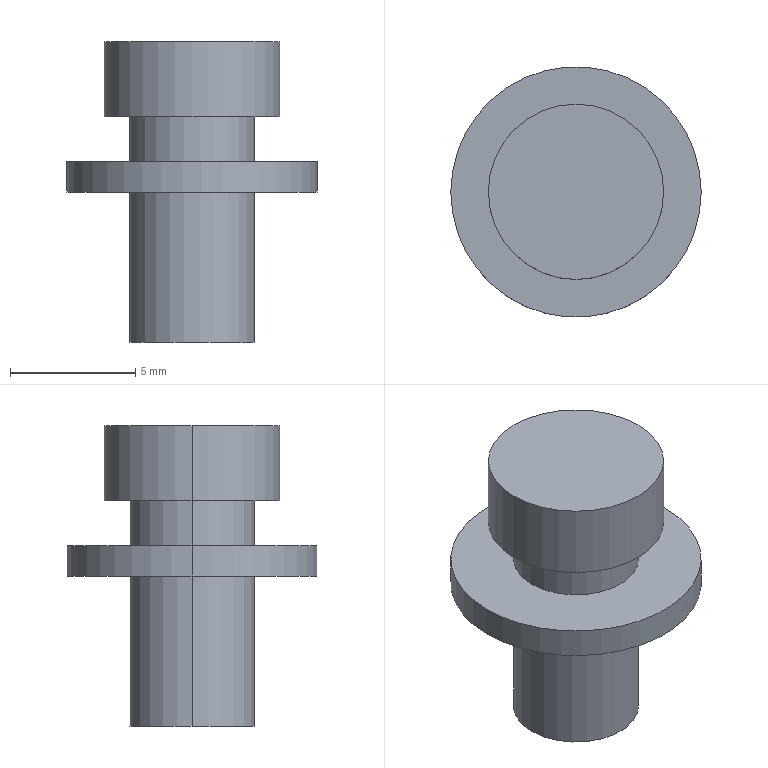Part | STEP file | 1 solid | 13 faces | box 10 x 10 x 12 mm | volume 362.854 mm3 | cylinder 8 | plane 5 | commonest cylinder face diameters 5 x4 7 x2 10 x2
STEP:
#1=CARTESIAN_POINT('',(0.,0.,0.));
#2=DIRECTION('',(0.,0.,1.));
#3=DIRECTION('',(1.,0.,0.));
#4=AXIS2_PLACEMENT_3D('',#1,#2,#3);
#5=CARTESIAN_POINT('',(2.5,0.,-11.));
#6=VERTEX_POINT('',#5);
#7=CARTESIAN_POINT('',(-2.5,0.,-11.));
#8=VERTEX_POINT('',#7);
#9=CARTESIAN_POINT('',(0.,0.,-11.));
#10=DIRECTION('',(0.,0.,-1.));
#11=DIRECTION('',(-1.,0.,0.));
#12=AXIS2_PLACEMENT_3D('',#9,#10,#11);
#13=CIRCLE('',#12,2.5);
#14=CARTESIAN_POINT('',(0.,0.,-11.));
#15=DIRECTION('',(0.,0.,-1.));
#16=DIRECTION('',(0.,-1.,0.));
#17=AXIS2_PLACEMENT_3D('',#14,#15,#16);
#18=PLANE('',#17);
#19=CARTESIAN_POINT('',(0.,0.));
#20=DIRECTION('',(0.,1.));
#21=AXIS2_PLACEMENT_2D('',#19,#20);
#22=CIRCLE('',#21,2.5);
#23=(GEOMETRIC_REPRESENTATION_CONTEXT(2)PARAMETRIC_REPRESENTATION_CONTEXT()REPRESENTATION_CONTEXT('',''));
#24=DEFINITIONAL_REPRESENTATION('',(#22),#23);
#25=PCURVE('',#18,#24);
#26=CARTESIAN_POINT('',(0.,0.,-6.));
#27=DIRECTION('',(0.,0.,1.));
#28=DIRECTION('',(1.,0.,0.));
#29=AXIS2_PLACEMENT_3D('',#26,#27,#28);
#30=CYLINDRICAL_SURFACE('',#29,2.5);
#31=CARTESIAN_POINT('',(9.425,-5.));
#32=DIRECTION('',(-1.,0.));
#33=VECTOR('',#32,1.);
#34=LINE('',#31,#33);
#35=(GEOMETRIC_REPRESENTATION_CONTEXT(2)PARAMETRIC_REPRESENTATION_CONTEXT()REPRESENTATION_CONTEXT('',''));
#36=DEFINITIONAL_REPRESENTATION('',(#34),#35);
#37=PCURVE('',#30,#36);
#38=SURFACE_CURVE('',#13,(#25,#37),.PCURVE_S1.);
#39=EDGE_CURVE('',#6,#8,#38,.T.);
#40=ORIENTED_EDGE('',*,*,#39,.T.);
#41=CARTESIAN_POINT('',(0.,0.,-11.));
#42=DIRECTION('',(0.,0.,-1.));
#43=DIRECTION('',(-1.,0.,0.));
#44=AXIS2_PLACEMENT_3D('',#41,#42,#43);
#45=CIRCLE('',#44,2.5);
#46=CARTESIAN_POINT('',(0.,0.));
#47=DIRECTION('',(0.,1.));
#48=AXIS2_PLACEMENT_2D('',#46,#47);
#49=CIRCLE('',#48,2.5);
#50=(GEOMETRIC_REPRESENTATION_CONTEXT(2)PARAMETRIC_REPRESENTATION_CONTEXT()REPRESENTATION_CONTEXT('',''));
#51=DEFINITIONAL_REPRESENTATION('',(#49),#50);
#52=PCURVE('',#18,#51);
#53=CARTESIAN_POINT('',(0.,0.,-6.));
#54=DIRECTION('',(0.,0.,1.));
#55=DIRECTION('',(1.,0.,0.));
#56=AXIS2_PLACEMENT_3D('',#53,#54,#55);
#57=CYLINDRICAL_SURFACE('',#56,2.5);
#58=CARTESIAN_POINT('',(3.142,-5.));
#59=DIRECTION('',(-1.,0.));
#60=VECTOR('',#59,1.);
#61=LINE('',#58,#60);
#62=(GEOMETRIC_REPRESENTATION_CONTEXT(2)PARAMETRIC_REPRESENTATION_CONTEXT()REPRESENTATION_CONTEXT('',''));
#63=DEFINITIONAL_REPRESENTATION('',(#61),#62);
#64=PCURVE('',#57,#63);
#65=SURFACE_CURVE('',#45,(#52,#64),.PCURVE_S1.);
#66=EDGE_CURVE('',#8,#6,#65,.T.);
#67=ORIENTED_EDGE('',*,*,#66,.T.);
#68=EDGE_LOOP('',(#40,#67));
#69=FACE_BOUND('',#68,.T.);
#70=ADVANCED_FACE('',(#69),#18,.T.);
#71=CARTESIAN_POINT('',(-2.5,0.,-5.));
#72=VERTEX_POINT('',#71);
#73=CARTESIAN_POINT('',(-2.5,0.,-6.));
#74=DIRECTION('',(0.,0.,1.));
#75=VECTOR('',#74,1.);
#76=LINE('',#73,#75);
#77=CARTESIAN_POINT('',(3.142,0.));
#78=DIRECTION('',(0.,1.));
#79=VECTOR('',#78,1.);
#80=LINE('',#77,#79);
#81=(GEOMETRIC_REPRESENTATION_CONTEXT(2)PARAMETRIC_REPRESENTATION_CONTEXT()REPRESENTATION_CONTEXT('',''));
#82=DEFINITIONAL_REPRESENTATION('',(#80),#81);
#83=PCURVE('',#30,#82);
#84=CARTESIAN_POINT('',(3.142,0.));
#85=DIRECTION('',(0.,1.));
#86=VECTOR('',#85,1.);
#87=LINE('',#84,#86);
#88=(GEOMETRIC_REPRESENTATION_CONTEXT(2)PARAMETRIC_REPRESENTATION_CONTEXT()REPRESENTATION_CONTEXT('',''));
#89=DEFINITIONAL_REPRESENTATION('',(#87),#88);
#90=PCURVE('',#57,#89);
#91=SURFACE_CURVE('',#76,(#83,#90),.PCURVE_S1.);
#92=EDGE_CURVE('',#8,#72,#91,.T.);
#93=ORIENTED_EDGE('',*,*,#92,.F.);
#94=ORIENTED_EDGE('',*,*,#39,.F.);
#95=CARTESIAN_POINT('',(2.5,0.,-5.));
#96=VERTEX_POINT('',#95);
#97=CARTESIAN_POINT('',(2.5,0.,-6.));
#98=DIRECTION('',(0.,0.,1.));
#99=VECTOR('',#98,1.);
#100=LINE('',#97,#99);
#101=CARTESIAN_POINT('',(6.283,0.));
#102=DIRECTION('',(0.,1.));
#103=VECTOR('',#102,1.);
#104=LINE('',#101,#103);
#105=(GEOMETRIC_REPRESENTATION_CONTEXT(2)PARAMETRIC_REPRESENTATION_CONTEXT()REPRESENTATION_CONTEXT('',''));
#106=DEFINITIONAL_REPRESENTATION('',(#104),#105);
#107=PCURVE('',#30,#106);
#108=CARTESIAN_POINT('',(0.,0.));
#109=DIRECTION('',(0.,1.));
#110=VECTOR('',#109,1.);
#111=LINE('',#108,#110);
#112=(GEOMETRIC_REPRESENTATION_CONTEXT(2)PARAMETRIC_REPRESENTATION_CONTEXT()REPRESENTATION_CONTEXT('',''));
#113=DEFINITIONAL_REPRESENTATION('',(#111),#112);
#114=PCURVE('',#57,#113);
#115=SURFACE_CURVE('',#100,(#107,#114),.PCURVE_S1.);
#116=EDGE_CURVE('',#6,#96,#115,.T.);
#117=ORIENTED_EDGE('',*,*,#116,.T.);
#118=CARTESIAN_POINT('',(0.,0.,-5.));
#119=DIRECTION('',(0.,0.,-1.));
#120=DIRECTION('',(1.,0.,0.));
#121=AXIS2_PLACEMENT_3D('',#118,#119,#120);
#122=CIRCLE('',#121,2.5);
#123=CARTESIAN_POINT('',(6.283,1.));
#124=DIRECTION('',(-1.,0.));
#125=VECTOR('',#124,1.);
#126=LINE('',#123,#125);
#127=(GEOMETRIC_REPRESENTATION_CONTEXT(2)PARAMETRIC_REPRESENTATION_CONTEXT()REPRESENTATION_CONTEXT('',''));
#128=DEFINITIONAL_REPRESENTATION('',(#126),#127);
#129=PCURVE('',#30,#128);
#130=CARTESIAN_POINT('',(0.,0.,-5.));
#131=DIRECTION('',(0.,0.,1.));
#132=DIRECTION('',(1.,0.,0.));
#133=AXIS2_PLACEMENT_3D('',#130,#131,#132);
#134=PLANE('',#133);
#135=CARTESIAN_POINT('',(2.5,0.));
#136=CARTESIAN_POINT('',(2.5,-4.33));
#137=CARTESIAN_POINT('',(-1.25,-2.165));
#138=CARTESIAN_POINT('',(-5.,0.));
#139=CARTESIAN_POINT('',(-1.25,2.165));
#140=CARTESIAN_POINT('',(2.5,4.33));
#141=CARTESIAN_POINT('',(2.5,0.));
#142=(BOUNDED_CURVE()B_SPLINE_CURVE(2,(#135,#136,#137,#138,#139,#140,#141),.UNSPECIFIED.,.T.,.F.)B_SPLINE_CURVE_WITH_KNOTS((1,2,2,2,2,1),(-2.094,0.,2.094,4.189,6.283,8.378),.UNSPECIFIED.)CURVE()GEOMETRIC_REPRESENTATION_ITEM()RATIONAL_B_SPLINE_CURVE((1.,0.5,1.,0.5,1.,0.5,1.))REPRESENTATION_ITEM(''));
#143=(GEOMETRIC_REPRESENTATION_CONTEXT(2)PARAMETRIC_REPRESENTATION_CONTEXT()REPRESENTATION_CONTEXT('',''));
#144=DEFINITIONAL_REPRESENTATION('',(#142),#143);
#145=PCURVE('',#134,#144);
#146=SURFACE_CURVE('',#122,(#129,#145),.PCURVE_S1.);
#147=EDGE_CURVE('',#96,#72,#146,.T.);
#148=ORIENTED_EDGE('',*,*,#147,.T.);
#149=EDGE_LOOP('',(#93,#94,#117,#148));
#150=FACE_BOUND('',#149,.T.);
#151=ADVANCED_FACE('',(#150),#30,.T.);
#152=ORIENTED_EDGE('',*,*,#147,.F.);
#153=CARTESIAN_POINT('',(0.,0.,-5.));
#154=DIRECTION('',(0.,0.,-1.));
#155=DIRECTION('',(1.,0.,0.));
#156=AXIS2_PLACEMENT_3D('',#153,#154,#155);
#157=CIRCLE('',#156,2.5);
#158=CARTESIAN_POINT('',(2.5,0.));
#159=CARTESIAN_POINT('',(2.5,-4.33));
#160=CARTESIAN_POINT('',(-1.25,-2.165));
#161=CARTESIAN_POINT('',(-5.,0.));
#162=CARTESIAN_POINT('',(-1.25,2.165));
#163=CARTESIAN_POINT('',(2.5,4.33));
#164=CARTESIAN_POINT('',(2.5,0.));
#165=(BOUNDED_CURVE()B_SPLINE_CURVE(2,(#158,#159,#160,#161,#162,#163,#164),.UNSPECIFIED.,.T.,.F.)B_SPLINE_CURVE_WITH_KNOTS((1,2,2,2,2,1),(-2.094,0.,2.094,4.189,6.283,8.378),.UNSPECIFIED.)CURVE()GEOMETRIC_REPRESENTATION_ITEM()RATIONAL_B_SPLINE_CURVE((1.,0.5,1.,0.5,1.,0.5,1.))REPRESENTATION_ITEM(''));
#166=(GEOMETRIC_REPRESENTATION_CONTEXT(2)PARAMETRIC_REPRESENTATION_CONTEXT()REPRESENTATION_CONTEXT('',''));
#167=DEFINITIONAL_REPRESENTATION('',(#165),#166);
#168=PCURVE('',#134,#167);
#169=CARTESIAN_POINT('',(6.283,1.));
#170=DIRECTION('',(-1.,0.));
#171=VECTOR('',#170,1.);
#172=LINE('',#169,#171);
#173=(GEOMETRIC_REPRESENTATION_CONTEXT(2)PARAMETRIC_REPRESENTATION_CONTEXT()REPRESENTATION_CONTEXT('',''));
#174=DEFINITIONAL_REPRESENTATION('',(#172),#173);
#175=PCURVE('',#57,#174);
#176=SURFACE_CURVE('',#157,(#168,#175),.PCURVE_S1.);
#177=EDGE_CURVE('',#72,#96,#176,.T.);
#178=ORIENTED_EDGE('',*,*,#177,.F.);
#179=EDGE_LOOP('',(#152,#178));
#180=FACE_BOUND('',#179,.T.);
#181=CARTESIAN_POINT('',(-5.,0.,-5.));
#182=VERTEX_POINT('',#181);
#183=CARTESIAN_POINT('',(5.,0.,-5.));
#184=VERTEX_POINT('',#183);
#185=CARTESIAN_POINT('',(0.,0.,-5.));
#186=DIRECTION('',(0.,0.,1.));
#187=DIRECTION('',(1.,0.,0.));
#188=AXIS2_PLACEMENT_3D('',#185,#186,#187);
#189=CIRCLE('',#188,5.);
#190=CARTESIAN_POINT('',(0.,0.));
#191=DIRECTION('',(1.,0.));
#192=AXIS2_PLACEMENT_2D('',#190,#191);
#193=CIRCLE('',#192,5.);
#194=(GEOMETRIC_REPRESENTATION_CONTEXT(2)PARAMETRIC_REPRESENTATION_CONTEXT()REPRESENTATION_CONTEXT('',''));
#195=DEFINITIONAL_REPRESENTATION('',(#193),#194);
#196=PCURVE('',#134,#195);
#197=CARTESIAN_POINT('',(0.,0.,35.));
#198=DIRECTION('',(0.,0.,-1.));
#199=DIRECTION('',(-1.,0.,0.));
#200=AXIS2_PLACEMENT_3D('',#197,#198,#199);
#201=CYLINDRICAL_SURFACE('',#200,5.);
#202=CARTESIAN_POINT('',(9.425,40.));
#203=DIRECTION('',(-1.,0.));
#204=VECTOR('',#203,1.);
#205=LINE('',#202,#204);
#206=(GEOMETRIC_REPRESENTATION_CONTEXT(2)PARAMETRIC_REPRESENTATION_CONTEXT()REPRESENTATION_CONTEXT('',''));
#207=DEFINITIONAL_REPRESENTATION('',(#205),#206);
#208=PCURVE('',#201,#207);
#209=SURFACE_CURVE('',#189,(#196,#208),.PCURVE_S1.);
#210=EDGE_CURVE('',#182,#184,#209,.T.);
#211=ORIENTED_EDGE('',*,*,#210,.F.);
#212=CARTESIAN_POINT('',(0.,0.,-5.));
#213=DIRECTION('',(0.,0.,1.));
#214=DIRECTION('',(1.,0.,0.));
#215=AXIS2_PLACEMENT_3D('',#212,#213,#214);
#216=CIRCLE('',#215,5.);
#217=CARTESIAN_POINT('',(0.,0.));
#218=DIRECTION('',(1.,0.));
#219=AXIS2_PLACEMENT_2D('',#217,#218);
#220=CIRCLE('',#219,5.);
#221=(GEOMETRIC_REPRESENTATION_CONTEXT(2)PARAMETRIC_REPRESENTATION_CONTEXT()REPRESENTATION_CONTEXT('',''));
#222=DEFINITIONAL_REPRESENTATION('',(#220),#221);
#223=PCURVE('',#134,#222);
#224=CARTESIAN_POINT('',(0.,0.,35.));
#225=DIRECTION('',(0.,0.,-1.));
#226=DIRECTION('',(-1.,0.,0.));
#227=AXIS2_PLACEMENT_3D('',#224,#225,#226);
#228=CYLINDRICAL_SURFACE('',#227,5.);
#229=CARTESIAN_POINT('',(3.142,40.));
#230=DIRECTION('',(-1.,0.));
#231=VECTOR('',#230,1.);
#232=LINE('',#229,#231);
#233=(GEOMETRIC_REPRESENTATION_CONTEXT(2)PARAMETRIC_REPRESENTATION_CONTEXT()REPRESENTATION_CONTEXT('',''));
#234=DEFINITIONAL_REPRESENTATION('',(#232),#233);
#235=PCURVE('',#228,#234);
#236=SURFACE_CURVE('',#216,(#223,#235),.PCURVE_S1.);
#237=EDGE_CURVE('',#184,#182,#236,.T.);
#238=ORIENTED_EDGE('',*,*,#237,.F.);
#239=EDGE_LOOP('',(#211,#238));
#240=FACE_BOUND('',#239,.T.);
#241=ADVANCED_FACE('',(#180,#240),#134,.F.);
#242=CARTESIAN_POINT('',(5.,0.,-3.8));
#243=VERTEX_POINT('',#242);
#244=CARTESIAN_POINT('',(5.,0.,35.));
#245=DIRECTION('',(0.,0.,-1.));
#246=VECTOR('',#245,1.);
#247=LINE('',#244,#246);
#248=CARTESIAN_POINT('',(3.142,0.));
#249=DIRECTION('',(0.,1.));
#250=VECTOR('',#249,1.);
#251=LINE('',#248,#250);
#252=(GEOMETRIC_REPRESENTATION_CONTEXT(2)PARAMETRIC_REPRESENTATION_CONTEXT()REPRESENTATION_CONTEXT('',''));
#253=DEFINITIONAL_REPRESENTATION('',(#251),#252);
#254=PCURVE('',#201,#253);
#255=CARTESIAN_POINT('',(3.142,0.));
#256=DIRECTION('',(0.,1.));
#257=VECTOR('',#256,1.);
#258=LINE('',#255,#257);
#259=(GEOMETRIC_REPRESENTATION_CONTEXT(2)PARAMETRIC_REPRESENTATION_CONTEXT()REPRESENTATION_CONTEXT('',''));
#260=DEFINITIONAL_REPRESENTATION('',(#258),#259);
#261=PCURVE('',#228,#260);
#262=SURFACE_CURVE('',#247,(#254,#261),.PCURVE_S1.);
#263=EDGE_CURVE('',#243,#184,#262,.T.);
#264=ORIENTED_EDGE('',*,*,#263,.F.);
#265=CARTESIAN_POINT('',(-5.,0.,-3.8));
#266=VERTEX_POINT('',#265);
#267=CARTESIAN_POINT('',(0.,0.,-3.8));
#268=DIRECTION('',(0.,0.,-1.));
#269=DIRECTION('',(1.,0.,0.));
#270=AXIS2_PLACEMENT_3D('',#267,#268,#269);
#271=CIRCLE('',#270,5.);
#272=CARTESIAN_POINT('',(3.142,38.8));
#273=DIRECTION('',(1.,0.));
#274=VECTOR('',#273,1.);
#275=LINE('',#272,#274);
#276=(GEOMETRIC_REPRESENTATION_CONTEXT(2)PARAMETRIC_REPRESENTATION_CONTEXT()REPRESENTATION_CONTEXT('',''));
#277=DEFINITIONAL_REPRESENTATION('',(#275),#276);
#278=PCURVE('',#201,#277);
#279=CARTESIAN_POINT('',(0.,0.,-3.8));
#280=DIRECTION('',(0.,0.,1.));
#281=DIRECTION('',(1.,0.,0.));
#282=AXIS2_PLACEMENT_3D('',#279,#280,#281);
#283=PLANE('',#282);
#284=CARTESIAN_POINT('',(5.,0.));
#285=CARTESIAN_POINT('',(5.,-8.66));
#286=CARTESIAN_POINT('',(-2.5,-4.33));
#287=CARTESIAN_POINT('',(-10.,0.));
#288=CARTESIAN_POINT('',(-2.5,4.33));
#289=CARTESIAN_POINT('',(5.,8.66));
#290=CARTESIAN_POINT('',(5.,0.));
#291=(BOUNDED_CURVE()B_SPLINE_CURVE(2,(#284,#285,#286,#287,#288,#289,#290),.UNSPECIFIED.,.T.,.F.)B_SPLINE_CURVE_WITH_KNOTS((1,2,2,2,2,1),(-2.094,0.,2.094,4.189,6.283,8.378),.UNSPECIFIED.)CURVE()GEOMETRIC_REPRESENTATION_ITEM()RATIONAL_B_SPLINE_CURVE((1.,0.5,1.,0.5,1.,0.5,1.))REPRESENTATION_ITEM(''));
#292=(GEOMETRIC_REPRESENTATION_CONTEXT(2)PARAMETRIC_REPRESENTATION_CONTEXT()REPRESENTATION_CONTEXT('',''));
#293=DEFINITIONAL_REPRESENTATION('',(#291),#292);
#294=PCURVE('',#283,#293);
#295=SURFACE_CURVE('',#271,(#278,#294),.PCURVE_S1.);
#296=EDGE_CURVE('',#243,#266,#295,.T.);
#297=ORIENTED_EDGE('',*,*,#296,.T.);
#298=CARTESIAN_POINT('',(-5.,0.,35.));
#299=DIRECTION('',(0.,0.,-1.));
#300=VECTOR('',#299,1.);
#301=LINE('',#298,#300);
#302=CARTESIAN_POINT('',(6.283,0.));
#303=DIRECTION('',(0.,1.));
#304=VECTOR('',#303,1.);
#305=LINE('',#302,#304);
#306=(GEOMETRIC_REPRESENTATION_CONTEXT(2)PARAMETRIC_REPRESENTATION_CONTEXT()REPRESENTATION_CONTEXT('',''));
#307=DEFINITIONAL_REPRESENTATION('',(#305),#306);
#308=PCURVE('',#201,#307);
#309=CARTESIAN_POINT('',(0.,0.));
#310=DIRECTION('',(0.,1.));
#311=VECTOR('',#310,1.);
#312=LINE('',#309,#311);
#313=(GEOMETRIC_REPRESENTATION_CONTEXT(2)PARAMETRIC_REPRESENTATION_CONTEXT()REPRESENTATION_CONTEXT('',''));
#314=DEFINITIONAL_REPRESENTATION('',(#312),#313);
#315=PCURVE('',#228,#314);
#316=SURFACE_CURVE('',#301,(#308,#315),.PCURVE_S1.);
#317=EDGE_CURVE('',#266,#182,#316,.T.);
#318=ORIENTED_EDGE('',*,*,#317,.T.);
#319=ORIENTED_EDGE('',*,*,#210,.T.);
#320=EDGE_LOOP('',(#264,#297,#318,#319));
#321=FACE_BOUND('',#320,.T.);
#322=ADVANCED_FACE('',(#321),#201,.T.);
#323=CARTESIAN_POINT('',(-2.5,0.,-2.));
#324=VERTEX_POINT('',#323);
#325=CARTESIAN_POINT('',(2.5,0.,-2.));
#326=VERTEX_POINT('',#325);
#327=CARTESIAN_POINT('',(0.,0.,-2.));
#328=DIRECTION('',(0.,0.,-1.));
#329=DIRECTION('',(-1.,0.,0.));
#330=AXIS2_PLACEMENT_3D('',#327,#328,#329);
#331=CIRCLE('',#330,2.5);
#332=CARTESIAN_POINT('',(0.,0.,-2.));
#333=DIRECTION('',(0.,0.,-1.));
#334=DIRECTION('',(-1.,0.,0.));
#335=AXIS2_PLACEMENT_3D('',#332,#333,#334);
#336=PLANE('',#335);
#337=CARTESIAN_POINT('',(0.,0.));
#338=DIRECTION('',(1.,0.));
#339=AXIS2_PLACEMENT_2D('',#337,#338);
#340=CIRCLE('',#339,2.5);
#341=(GEOMETRIC_REPRESENTATION_CONTEXT(2)PARAMETRIC_REPRESENTATION_CONTEXT()REPRESENTATION_CONTEXT('',''));
#342=DEFINITIONAL_REPRESENTATION('',(#340),#341);
#343=PCURVE('',#336,#342);
#344=CARTESIAN_POINT('',(0.,0.,1.));
#345=DIRECTION('',(0.,0.,-1.));
#346=DIRECTION('',(-1.,0.,0.));
#347=AXIS2_PLACEMENT_3D('',#344,#345,#346);
#348=CYLINDRICAL_SURFACE('',#347,2.5);
#349=CARTESIAN_POINT('',(0.,3.));
#350=DIRECTION('',(1.,0.));
#351=VECTOR('',#350,1.);
#352=LINE('',#349,#351);
#353=(GEOMETRIC_REPRESENTATION_CONTEXT(2)PARAMETRIC_REPRESENTATION_CONTEXT()REPRESENTATION_CONTEXT('',''));
#354=DEFINITIONAL_REPRESENTATION('',(#352),#353);
#355=PCURVE('',#348,#354);
#356=SURFACE_CURVE('',#331,(#343,#355),.PCURVE_S1.);
#357=EDGE_CURVE('',#324,#326,#356,.T.);
#358=ORIENTED_EDGE('',*,*,#357,.F.);
#359=CARTESIAN_POINT('',(0.,0.,-2.));
#360=DIRECTION('',(0.,0.,-1.));
#361=DIRECTION('',(-1.,0.,0.));
#362=AXIS2_PLACEMENT_3D('',#359,#360,#361);
#363=CIRCLE('',#362,2.5);
#364=CARTESIAN_POINT('',(0.,0.));
#365=DIRECTION('',(1.,0.));
#366=AXIS2_PLACEMENT_2D('',#364,#365);
#367=CIRCLE('',#366,2.5);
#368=(GEOMETRIC_REPRESENTATION_CONTEXT(2)PARAMETRIC_REPRESENTATION_CONTEXT()REPRESENTATION_CONTEXT('',''));
#369=DEFINITIONAL_REPRESENTATION('',(#367),#368);
#370=PCURVE('',#336,#369);
#371=CARTESIAN_POINT('',(0.,0.,1.));
#372=DIRECTION('',(0.,0.,-1.));
#373=DIRECTION('',(-1.,0.,0.));
#374=AXIS2_PLACEMENT_3D('',#371,#372,#373);
#375=CYLINDRICAL_SURFACE('',#374,2.5);
#376=CARTESIAN_POINT('',(0.,3.));
#377=DIRECTION('',(1.,0.));
#378=VECTOR('',#377,1.);
#379=LINE('',#376,#378);
#380=(GEOMETRIC_REPRESENTATION_CONTEXT(2)PARAMETRIC_REPRESENTATION_CONTEXT()REPRESENTATION_CONTEXT('',''));
#381=DEFINITIONAL_REPRESENTATION('',(#379),#380);
#382=PCURVE('',#375,#381);
#383=SURFACE_CURVE('',#363,(#370,#382),.PCURVE_S1.);
#384=EDGE_CURVE('',#326,#324,#383,.T.);
#385=ORIENTED_EDGE('',*,*,#384,.F.);
#386=EDGE_LOOP('',(#358,#385));
#387=FACE_BOUND('',#386,.T.);
#388=CARTESIAN_POINT('',(-3.5,0.,-2.));
#389=VERTEX_POINT('',#388);
#390=CARTESIAN_POINT('',(3.5,0.,-2.));
#391=VERTEX_POINT('',#390);
#392=CARTESIAN_POINT('',(0.,0.,-2.));
#393=DIRECTION('',(0.,0.,-1.));
#394=DIRECTION('',(-1.,0.,0.));
#395=AXIS2_PLACEMENT_3D('',#392,#393,#394);
#396=CIRCLE('',#395,3.5);
#397=CARTESIAN_POINT('',(0.,0.));
#398=DIRECTION('',(1.,0.));
#399=AXIS2_PLACEMENT_2D('',#397,#398);
#400=CIRCLE('',#399,3.5);
#401=(GEOMETRIC_REPRESENTATION_CONTEXT(2)PARAMETRIC_REPRESENTATION_CONTEXT()REPRESENTATION_CONTEXT('',''));
#402=DEFINITIONAL_REPRESENTATION('',(#400),#401);
#403=PCURVE('',#336,#402);
#404=CARTESIAN_POINT('',(0.,0.,1.));
#405=DIRECTION('',(0.,0.,-1.));
#406=DIRECTION('',(-1.,0.,0.));
#407=AXIS2_PLACEMENT_3D('',#404,#405,#406);
#408=CYLINDRICAL_SURFACE('',#407,3.5);
#409=CARTESIAN_POINT('',(0.,3.));
#410=DIRECTION('',(1.,0.));
#411=VECTOR('',#410,1.);
#412=LINE('',#409,#411);
#413=(GEOMETRIC_REPRESENTATION_CONTEXT(2)PARAMETRIC_REPRESENTATION_CONTEXT()REPRESENTATION_CONTEXT('',''));
#414=DEFINITIONAL_REPRESENTATION('',(#412),#413);
#415=PCURVE('',#408,#414);
#416=SURFACE_CURVE('',#396,(#403,#415),.PCURVE_S1.);
#417=EDGE_CURVE('',#389,#391,#416,.T.);
#418=ORIENTED_EDGE('',*,*,#417,.T.);
#419=CARTESIAN_POINT('',(0.,0.,-2.));
#420=DIRECTION('',(0.,0.,-1.));
#421=DIRECTION('',(-1.,0.,0.));
#422=AXIS2_PLACEMENT_3D('',#419,#420,#421);
#423=CIRCLE('',#422,3.5);
#424=CARTESIAN_POINT('',(0.,0.));
#425=DIRECTION('',(1.,0.));
#426=AXIS2_PLACEMENT_2D('',#424,#425);
#427=CIRCLE('',#426,3.5);
#428=(GEOMETRIC_REPRESENTATION_CONTEXT(2)PARAMETRIC_REPRESENTATION_CONTEXT()REPRESENTATION_CONTEXT('',''));
#429=DEFINITIONAL_REPRESENTATION('',(#427),#428);
#430=PCURVE('',#336,#429);
#431=CARTESIAN_POINT('',(0.,0.,1.));
#432=DIRECTION('',(0.,0.,-1.));
#433=DIRECTION('',(-1.,0.,0.));
#434=AXIS2_PLACEMENT_3D('',#431,#432,#433);
#435=CYLINDRICAL_SURFACE('',#434,3.5);
#436=CARTESIAN_POINT('',(0.,3.));
#437=DIRECTION('',(1.,0.));
#438=VECTOR('',#437,1.);
#439=LINE('',#436,#438);
#440=(GEOMETRIC_REPRESENTATION_CONTEXT(2)PARAMETRIC_REPRESENTATION_CONTEXT()REPRESENTATION_CONTEXT('',''));
#441=DEFINITIONAL_REPRESENTATION('',(#439),#440);
#442=PCURVE('',#435,#441);
#443=SURFACE_CURVE('',#423,(#430,#442),.PCURVE_S1.);
#444=EDGE_CURVE('',#391,#389,#443,.T.);
#445=ORIENTED_EDGE('',*,*,#444,.T.);
#446=EDGE_LOOP('',(#418,#445));
#447=FACE_BOUND('',#446,.T.);
#448=ADVANCED_FACE('',(#387,#447),#336,.T.);
#449=CARTESIAN_POINT('',(2.5,0.,-3.8));
#450=VERTEX_POINT('',#449);
#451=CARTESIAN_POINT('',(2.5,0.,1.));
#452=DIRECTION('',(0.,0.,-1.));
#453=VECTOR('',#452,1.);
#454=LINE('',#451,#453);
#455=CARTESIAN_POINT('',(3.142,0.));
#456=DIRECTION('',(0.,1.));
#457=VECTOR('',#456,1.);
#458=LINE('',#455,#457);
#459=(GEOMETRIC_REPRESENTATION_CONTEXT(2)PARAMETRIC_REPRESENTATION_CONTEXT()REPRESENTATION_CONTEXT('',''));
#460=DEFINITIONAL_REPRESENTATION('',(#458),#459);
#461=PCURVE('',#375,#460);
#462=CARTESIAN_POINT('',(3.142,0.));
#463=DIRECTION('',(0.,1.));
#464=VECTOR('',#463,1.);
#465=LINE('',#462,#464);
#466=(GEOMETRIC_REPRESENTATION_CONTEXT(2)PARAMETRIC_REPRESENTATION_CONTEXT()REPRESENTATION_CONTEXT('',''));
#467=DEFINITIONAL_REPRESENTATION('',(#465),#466);
#468=PCURVE('',#348,#467);
#469=SURFACE_CURVE('',#454,(#461,#468),.PCURVE_S1.);
#470=EDGE_CURVE('',#326,#450,#469,.T.);
#471=ORIENTED_EDGE('',*,*,#470,.F.);
#472=ORIENTED_EDGE('',*,*,#384,.T.);
#473=CARTESIAN_POINT('',(-2.5,0.,-3.8));
#474=VERTEX_POINT('',#473);
#475=CARTESIAN_POINT('',(-2.5,0.,1.));
#476=DIRECTION('',(0.,0.,-1.));
#477=VECTOR('',#476,1.);
#478=LINE('',#475,#477);
#479=CARTESIAN_POINT('',(6.283,0.));
#480=DIRECTION('',(0.,1.));
#481=VECTOR('',#480,1.);
#482=LINE('',#479,#481);
#483=(GEOMETRIC_REPRESENTATION_CONTEXT(2)PARAMETRIC_REPRESENTATION_CONTEXT()REPRESENTATION_CONTEXT('',''));
#484=DEFINITIONAL_REPRESENTATION('',(#482),#483);
#485=PCURVE('',#375,#484);
#486=CARTESIAN_POINT('',(0.,0.));
#487=DIRECTION('',(0.,1.));
#488=VECTOR('',#487,1.);
#489=LINE('',#486,#488);
#490=(GEOMETRIC_REPRESENTATION_CONTEXT(2)PARAMETRIC_REPRESENTATION_CONTEXT()REPRESENTATION_CONTEXT('',''));
#491=DEFINITIONAL_REPRESENTATION('',(#489),#490);
#492=PCURVE('',#348,#491);
#493=SURFACE_CURVE('',#478,(#485,#492),.PCURVE_S1.);
#494=EDGE_CURVE('',#324,#474,#493,.T.);
#495=ORIENTED_EDGE('',*,*,#494,.T.);
#496=CARTESIAN_POINT('',(0.,0.,-3.8));
#497=DIRECTION('',(0.,0.,-1.));
#498=DIRECTION('',(-1.,0.,0.));
#499=AXIS2_PLACEMENT_3D('',#496,#497,#498);
#500=CIRCLE('',#499,2.5);
#501=CARTESIAN_POINT('',(0.,4.8));
#502=DIRECTION('',(1.,0.));
#503=VECTOR('',#502,1.);
#504=LINE('',#501,#503);
#505=(GEOMETRIC_REPRESENTATION_CONTEXT(2)PARAMETRIC_REPRESENTATION_CONTEXT()REPRESENTATION_CONTEXT('',''));
#506=DEFINITIONAL_REPRESENTATION('',(#504),#505);
#507=PCURVE('',#375,#506);
#508=CARTESIAN_POINT('',(-2.5,0.));
#509=CARTESIAN_POINT('',(-2.5,4.33));
#510=CARTESIAN_POINT('',(1.25,2.165));
#511=CARTESIAN_POINT('',(5.,0.));
#512=CARTESIAN_POINT('',(1.25,-2.165));
#513=CARTESIAN_POINT('',(-2.5,-4.33));
#514=CARTESIAN_POINT('',(-2.5,0.));
#515=(BOUNDED_CURVE()B_SPLINE_CURVE(2,(#508,#509,#510,#511,#512,#513,#514),.UNSPECIFIED.,.T.,.F.)B_SPLINE_CURVE_WITH_KNOTS((1,2,2,2,2,1),(-2.094,0.,2.094,4.189,6.283,8.378),.UNSPECIFIED.)CURVE()GEOMETRIC_REPRESENTATION_ITEM()RATIONAL_B_SPLINE_CURVE((1.,0.5,1.,0.5,1.,0.5,1.))REPRESENTATION_ITEM(''));
#516=(GEOMETRIC_REPRESENTATION_CONTEXT(2)PARAMETRIC_REPRESENTATION_CONTEXT()REPRESENTATION_CONTEXT('',''));
#517=DEFINITIONAL_REPRESENTATION('',(#515),#516);
#518=PCURVE('',#283,#517);
#519=SURFACE_CURVE('',#500,(#507,#518),.PCURVE_S1.);
#520=EDGE_CURVE('',#450,#474,#519,.T.);
#521=ORIENTED_EDGE('',*,*,#520,.F.);
#522=EDGE_LOOP('',(#471,#472,#495,#521));
#523=FACE_BOUND('',#522,.T.);
#524=ADVANCED_FACE('',(#523),#375,.T.);
#525=CARTESIAN_POINT('',(0.,0.,-3.8));
#526=DIRECTION('',(0.,0.,-1.));
#527=DIRECTION('',(-1.,0.,0.));
#528=AXIS2_PLACEMENT_3D('',#525,#526,#527);
#529=CIRCLE('',#528,2.5);
#530=CARTESIAN_POINT('',(-2.5,0.));
#531=CARTESIAN_POINT('',(-2.5,4.33));
#532=CARTESIAN_POINT('',(1.25,2.165));
#533=CARTESIAN_POINT('',(5.,0.));
#534=CARTESIAN_POINT('',(1.25,-2.165));
#535=CARTESIAN_POINT('',(-2.5,-4.33));
#536=CARTESIAN_POINT('',(-2.5,0.));
#537=(BOUNDED_CURVE()B_SPLINE_CURVE(2,(#530,#531,#532,#533,#534,#535,#536),.UNSPECIFIED.,.T.,.F.)B_SPLINE_CURVE_WITH_KNOTS((1,2,2,2,2,1),(-2.094,0.,2.094,4.189,6.283,8.378),.UNSPECIFIED.)CURVE()GEOMETRIC_REPRESENTATION_ITEM()RATIONAL_B_SPLINE_CURVE((1.,0.5,1.,0.5,1.,0.5,1.))REPRESENTATION_ITEM(''));
#538=(GEOMETRIC_REPRESENTATION_CONTEXT(2)PARAMETRIC_REPRESENTATION_CONTEXT()REPRESENTATION_CONTEXT('',''));
#539=DEFINITIONAL_REPRESENTATION('',(#537),#538);
#540=PCURVE('',#283,#539);
#541=CARTESIAN_POINT('',(0.,4.8));
#542=DIRECTION('',(1.,0.));
#543=VECTOR('',#542,1.);
#544=LINE('',#541,#543);
#545=(GEOMETRIC_REPRESENTATION_CONTEXT(2)PARAMETRIC_REPRESENTATION_CONTEXT()REPRESENTATION_CONTEXT('',''));
#546=DEFINITIONAL_REPRESENTATION('',(#544),#545);
#547=PCURVE('',#348,#546);
#548=SURFACE_CURVE('',#529,(#540,#547),.PCURVE_S1.);
#549=EDGE_CURVE('',#474,#450,#548,.T.);
#550=ORIENTED_EDGE('',*,*,#549,.T.);
#551=ORIENTED_EDGE('',*,*,#520,.T.);
#552=EDGE_LOOP('',(#550,#551));
#553=FACE_BOUND('',#552,.T.);
#554=CARTESIAN_POINT('',(0.,0.,-3.8));
#555=DIRECTION('',(0.,0.,-1.));
#556=DIRECTION('',(1.,0.,0.));
#557=AXIS2_PLACEMENT_3D('',#554,#555,#556);
#558=CIRCLE('',#557,5.);
#559=CARTESIAN_POINT('',(5.,0.));
#560=CARTESIAN_POINT('',(5.,-8.66));
#561=CARTESIAN_POINT('',(-2.5,-4.33));
#562=CARTESIAN_POINT('',(-10.,0.));
#563=CARTESIAN_POINT('',(-2.5,4.33));
#564=CARTESIAN_POINT('',(5.,8.66));
#565=CARTESIAN_POINT('',(5.,0.));
#566=(BOUNDED_CURVE()B_SPLINE_CURVE(2,(#559,#560,#561,#562,#563,#564,#565),.UNSPECIFIED.,.T.,.F.)B_SPLINE_CURVE_WITH_KNOTS((1,2,2,2,2,1),(-2.094,0.,2.094,4.189,6.283,8.378),.UNSPECIFIED.)CURVE()GEOMETRIC_REPRESENTATION_ITEM()RATIONAL_B_SPLINE_CURVE((1.,0.5,1.,0.5,1.,0.5,1.))REPRESENTATION_ITEM(''));
#567=(GEOMETRIC_REPRESENTATION_CONTEXT(2)PARAMETRIC_REPRESENTATION_CONTEXT()REPRESENTATION_CONTEXT('',''));
#568=DEFINITIONAL_REPRESENTATION('',(#566),#567);
#569=PCURVE('',#283,#568);
#570=CARTESIAN_POINT('',(-3.142,38.8));
#571=DIRECTION('',(1.,0.));
#572=VECTOR('',#571,1.);
#573=LINE('',#570,#572);
#574=(GEOMETRIC_REPRESENTATION_CONTEXT(2)PARAMETRIC_REPRESENTATION_CONTEXT()REPRESENTATION_CONTEXT('',''));
#575=DEFINITIONAL_REPRESENTATION('',(#573),#574);
#576=PCURVE('',#228,#575);
#577=SURFACE_CURVE('',#558,(#569,#576),.PCURVE_S1.);
#578=EDGE_CURVE('',#266,#243,#577,.T.);
#579=ORIENTED_EDGE('',*,*,#578,.F.);
#580=ORIENTED_EDGE('',*,*,#296,.F.);
#581=EDGE_LOOP('',(#579,#580));
#582=FACE_BOUND('',#581,.T.);
#583=ADVANCED_FACE('',(#553,#582),#283,.T.);
#584=CARTESIAN_POINT('',(-3.5,0.,1.));
#585=VERTEX_POINT('',#584);
#586=CARTESIAN_POINT('',(3.5,0.,1.));
#587=VERTEX_POINT('',#586);
#588=CARTESIAN_POINT('',(0.,0.,1.));
#589=DIRECTION('',(0.,0.,-1.));
#590=DIRECTION('',(-1.,0.,0.));
#591=AXIS2_PLACEMENT_3D('',#588,#589,#590);
#592=CIRCLE('',#591,3.5);
#593=CARTESIAN_POINT('',(0.,0.,1.));
#594=DIRECTION('',(0.,0.,1.));
#595=DIRECTION('',(1.,0.,0.));
#596=AXIS2_PLACEMENT_3D('',#593,#594,#595);
#597=PLANE('',#596);
#598=CARTESIAN_POINT('',(-3.5,0.));
#599=CARTESIAN_POINT('',(-3.5,6.062));
#600=CARTESIAN_POINT('',(1.75,3.031));
#601=CARTESIAN_POINT('',(7.,0.));
#602=CARTESIAN_POINT('',(1.75,-3.031));
#603=CARTESIAN_POINT('',(-3.5,-6.062));
#604=CARTESIAN_POINT('',(-3.5,0.));
#605=(BOUNDED_CURVE()B_SPLINE_CURVE(2,(#598,#599,#600,#601,#602,#603,#604),.UNSPECIFIED.,.T.,.F.)B_SPLINE_CURVE_WITH_KNOTS((1,2,2,2,2,1),(-2.094,0.,2.094,4.189,6.283,8.378),.UNSPECIFIED.)CURVE()GEOMETRIC_REPRESENTATION_ITEM()RATIONAL_B_SPLINE_CURVE((1.,0.5,1.,0.5,1.,0.5,1.))REPRESENTATION_ITEM(''));
#606=(GEOMETRIC_REPRESENTATION_CONTEXT(2)PARAMETRIC_REPRESENTATION_CONTEXT()REPRESENTATION_CONTEXT('',''));
#607=DEFINITIONAL_REPRESENTATION('',(#605),#606);
#608=PCURVE('',#597,#607);
#609=CARTESIAN_POINT('',(0.,0.));
#610=DIRECTION('',(1.,0.));
#611=VECTOR('',#610,1.);
#612=LINE('',#609,#611);
#613=(GEOMETRIC_REPRESENTATION_CONTEXT(2)PARAMETRIC_REPRESENTATION_CONTEXT()REPRESENTATION_CONTEXT('',''));
#614=DEFINITIONAL_REPRESENTATION('',(#612),#613);
#615=PCURVE('',#408,#614);
#616=SURFACE_CURVE('',#592,(#608,#615),.PCURVE_S1.);
#617=EDGE_CURVE('',#585,#587,#616,.T.);
#618=ORIENTED_EDGE('',*,*,#617,.F.);
#619=CARTESIAN_POINT('',(0.,0.,1.));
#620=DIRECTION('',(0.,0.,-1.));
#621=DIRECTION('',(-1.,0.,0.));
#622=AXIS2_PLACEMENT_3D('',#619,#620,#621);
#623=CIRCLE('',#622,3.5);
#624=CARTESIAN_POINT('',(-3.5,0.));
#625=CARTESIAN_POINT('',(-3.5,6.062));
#626=CARTESIAN_POINT('',(1.75,3.031));
#627=CARTESIAN_POINT('',(7.,0.));
#628=CARTESIAN_POINT('',(1.75,-3.031));
#629=CARTESIAN_POINT('',(-3.5,-6.062));
#630=CARTESIAN_POINT('',(-3.5,0.));
#631=(BOUNDED_CURVE()B_SPLINE_CURVE(2,(#624,#625,#626,#627,#628,#629,#630),.UNSPECIFIED.,.T.,.F.)B_SPLINE_CURVE_WITH_KNOTS((1,2,2,2,2,1),(-2.094,0.,2.094,4.189,6.283,8.378),.UNSPECIFIED.)CURVE()GEOMETRIC_REPRESENTATION_ITEM()RATIONAL_B_SPLINE_CURVE((1.,0.5,1.,0.5,1.,0.5,1.))REPRESENTATION_ITEM(''));
#632=(GEOMETRIC_REPRESENTATION_CONTEXT(2)PARAMETRIC_REPRESENTATION_CONTEXT()REPRESENTATION_CONTEXT('',''));
#633=DEFINITIONAL_REPRESENTATION('',(#631),#632);
#634=PCURVE('',#597,#633);
#635=CARTESIAN_POINT('',(0.,0.));
#636=DIRECTION('',(1.,0.));
#637=VECTOR('',#636,1.);
#638=LINE('',#635,#637);
#639=(GEOMETRIC_REPRESENTATION_CONTEXT(2)PARAMETRIC_REPRESENTATION_CONTEXT()REPRESENTATION_CONTEXT('',''));
#640=DEFINITIONAL_REPRESENTATION('',(#638),#639);
#641=PCURVE('',#435,#640);
#642=SURFACE_CURVE('',#623,(#634,#641),.PCURVE_S1.);
#643=EDGE_CURVE('',#587,#585,#642,.T.);
#644=ORIENTED_EDGE('',*,*,#643,.F.);
#645=EDGE_LOOP('',(#618,#644));
#646=FACE_BOUND('',#645,.T.);
#647=ADVANCED_FACE('',(#646),#597,.T.);
#648=CARTESIAN_POINT('',(3.5,0.,1.));
#649=DIRECTION('',(0.,0.,-1.));
#650=VECTOR('',#649,1.);
#651=LINE('',#648,#650);
#652=CARTESIAN_POINT('',(3.142,0.));
#653=DIRECTION('',(0.,1.));
#654=VECTOR('',#653,1.);
#655=LINE('',#652,#654);
#656=(GEOMETRIC_REPRESENTATION_CONTEXT(2)PARAMETRIC_REPRESENTATION_CONTEXT()REPRESENTATION_CONTEXT('',''));
#657=DEFINITIONAL_REPRESENTATION('',(#655),#656);
#658=PCURVE('',#435,#657);
#659=CARTESIAN_POINT('',(3.142,0.));
#660=DIRECTION('',(0.,1.));
#661=VECTOR('',#660,1.);
#662=LINE('',#659,#661);
#663=(GEOMETRIC_REPRESENTATION_CONTEXT(2)PARAMETRIC_REPRESENTATION_CONTEXT()REPRESENTATION_CONTEXT('',''));
#664=DEFINITIONAL_REPRESENTATION('',(#662),#663);
#665=PCURVE('',#408,#664);
#666=SURFACE_CURVE('',#651,(#658,#665),.PCURVE_S1.);
#667=EDGE_CURVE('',#587,#391,#666,.T.);
#668=ORIENTED_EDGE('',*,*,#667,.F.);
#669=ORIENTED_EDGE('',*,*,#643,.T.);
#670=CARTESIAN_POINT('',(-3.5,0.,1.));
#671=DIRECTION('',(0.,0.,-1.));
#672=VECTOR('',#671,1.);
#673=LINE('',#670,#672);
#674=CARTESIAN_POINT('',(6.283,0.));
#675=DIRECTION('',(0.,1.));
#676=VECTOR('',#675,1.);
#677=LINE('',#674,#676);
#678=(GEOMETRIC_REPRESENTATION_CONTEXT(2)PARAMETRIC_REPRESENTATION_CONTEXT()REPRESENTATION_CONTEXT('',''));
#679=DEFINITIONAL_REPRESENTATION('',(#677),#678);
#680=PCURVE('',#435,#679);
#681=CARTESIAN_POINT('',(0.,0.));
#682=DIRECTION('',(0.,1.));
#683=VECTOR('',#682,1.);
#684=LINE('',#681,#683);
#685=(GEOMETRIC_REPRESENTATION_CONTEXT(2)PARAMETRIC_REPRESENTATION_CONTEXT()REPRESENTATION_CONTEXT('',''));
#686=DEFINITIONAL_REPRESENTATION('',(#684),#685);
#687=PCURVE('',#408,#686);
#688=SURFACE_CURVE('',#673,(#680,#687),.PCURVE_S1.);
#689=EDGE_CURVE('',#585,#389,#688,.T.);
#690=ORIENTED_EDGE('',*,*,#689,.T.);
#691=ORIENTED_EDGE('',*,*,#444,.F.);
#692=EDGE_LOOP('',(#668,#669,#690,#691));
#693=FACE_BOUND('',#692,.T.);
#694=ADVANCED_FACE('',(#693),#435,.T.);
#695=ORIENTED_EDGE('',*,*,#617,.T.);
#696=ORIENTED_EDGE('',*,*,#667,.T.);
#697=ORIENTED_EDGE('',*,*,#417,.F.);
#698=ORIENTED_EDGE('',*,*,#689,.F.);
#699=EDGE_LOOP('',(#695,#696,#697,#698));
#700=FACE_BOUND('',#699,.T.);
#701=ADVANCED_FACE('',(#700),#408,.T.);
#702=ORIENTED_EDGE('',*,*,#357,.T.);
#703=ORIENTED_EDGE('',*,*,#470,.T.);
#704=ORIENTED_EDGE('',*,*,#549,.F.);
#705=ORIENTED_EDGE('',*,*,#494,.F.);
#706=EDGE_LOOP('',(#702,#703,#704,#705));
#707=FACE_BOUND('',#706,.T.);
#708=ADVANCED_FACE('',(#707),#348,.T.);
#709=ORIENTED_EDGE('',*,*,#578,.T.);
#710=ORIENTED_EDGE('',*,*,#263,.T.);
#711=ORIENTED_EDGE('',*,*,#237,.T.);
#712=ORIENTED_EDGE('',*,*,#317,.F.);
#713=EDGE_LOOP('',(#709,#710,#711,#712));
#714=FACE_BOUND('',#713,.T.);
#715=ADVANCED_FACE('',(#714),#228,.T.);
#716=ORIENTED_EDGE('',*,*,#66,.F.);
#717=ORIENTED_EDGE('',*,*,#92,.T.);
#718=ORIENTED_EDGE('',*,*,#177,.T.);
#719=ORIENTED_EDGE('',*,*,#116,.F.);
#720=EDGE_LOOP('',(#716,#717,#718,#719));
#721=FACE_BOUND('',#720,.T.);
#722=ADVANCED_FACE('',(#721),#57,.T.);
#723=CLOSED_SHELL('',(#70,#151,#241,#322,#448,#524,#583,#647,#694,#701,#708,#715,#722));
#724=MANIFOLD_SOLID_BREP('',#723);
#725=(LENGTH_UNIT()NAMED_UNIT(*)SI_UNIT(.MILLI.,.METRE.));
#726=UNCERTAINTY_MEASURE_WITH_UNIT(LENGTH_MEASURE(0.0000001),#725,'','');
#727=(NAMED_UNIT(*)PLANE_ANGLE_UNIT()SI_UNIT($,.RADIAN.));
#728=(NAMED_UNIT(*)SI_UNIT($,.STERADIAN.)SOLID_ANGLE_UNIT());
#729=(GEOMETRIC_REPRESENTATION_CONTEXT(3)GLOBAL_UNCERTAINTY_ASSIGNED_CONTEXT((#726))GLOBAL_UNIT_ASSIGNED_CONTEXT((#725,#727,#728))REPRESENTATION_CONTEXT('',''));
#730=ADVANCED_BREP_SHAPE_REPRESENTATION('',(#4,#724),#729);